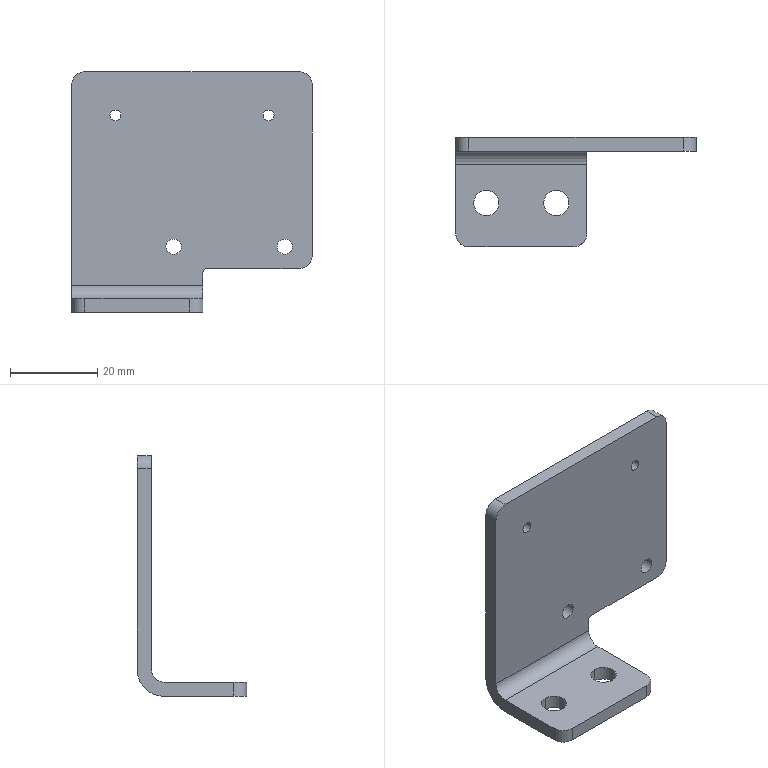Part | STEP file | J014-EBZ05-13-06-Part-1 | 1 solid | 30 faces | box 55 x 25 x 55 mm | volume 10507 mm3 | cylinder 20 | plane 10 | commonest cylinder face diameters 6 x6 2.5 x4 3.5 x4 5.8 x4 2 x1 12 x1
STEP:
#1=CARTESIAN_POINT('',(43.75,0.,45.));
#2=VERTEX_POINT('',#1);
#3=CARTESIAN_POINT('',(46.25,0.,45.));
#4=VERTEX_POINT('',#3);
#5=CARTESIAN_POINT('',(45.,0.,45.));
#6=DIRECTION('',(0.,-1.,0.));
#7=DIRECTION('',(1.,0.,0.));
#8=AXIS2_PLACEMENT_3D('',#5,#6,#7);
#9=CIRCLE('',#8,1.25);
#10=EDGE_CURVE('',#2,#4,#9,.T.);
#11=ORIENTED_EDGE('',*,*,#10,.F.);
#12=CARTESIAN_POINT('',(43.75,-3.2,45.));
#13=VERTEX_POINT('',#12);
#14=CARTESIAN_POINT('',(43.75,0.,45.));
#15=DIRECTION('',(0.,-1.,0.));
#16=VECTOR('',#15,1000.);
#17=LINE('',#14,#16);
#18=EDGE_CURVE('',#2,#13,#17,.T.);
#19=ORIENTED_EDGE('',*,*,#18,.T.);
#20=CARTESIAN_POINT('',(46.25,-3.2,45.));
#21=VERTEX_POINT('',#20);
#22=CARTESIAN_POINT('',(45.,-3.2,45.));
#23=DIRECTION('',(0.,1.,0.));
#24=DIRECTION('',(-1.,0.,0.));
#25=AXIS2_PLACEMENT_3D('',#22,#23,#24);
#26=CIRCLE('',#25,1.25);
#27=EDGE_CURVE('',#21,#13,#26,.T.);
#28=ORIENTED_EDGE('',*,*,#27,.F.);
#29=CARTESIAN_POINT('',(46.25,0.,45.));
#30=DIRECTION('',(0.,-1.,0.));
#31=VECTOR('',#30,1000.);
#32=LINE('',#29,#31);
#33=EDGE_CURVE('',#4,#21,#32,.T.);
#34=ORIENTED_EDGE('',*,*,#33,.F.);
#35=EDGE_LOOP('',(#11,#19,#28,#34));
#36=FACE_OUTER_BOUND('',#35,.T.);
#37=CARTESIAN_POINT('',(45.,0.,45.));
#38=DIRECTION('',(0.,-1.,0.));
#39=DIRECTION('',(1.,0.,0.));
#40=AXIS2_PLACEMENT_3D('',#37,#38,#39);
#41=CYLINDRICAL_SURFACE('',#40,1.25);
#42=ADVANCED_FACE('',(#36),#41,.F.);
#43=CARTESIAN_POINT('',(8.75,0.,45.));
#44=VERTEX_POINT('',#43);
#45=CARTESIAN_POINT('',(11.25,0.,45.));
#46=VERTEX_POINT('',#45);
#47=CARTESIAN_POINT('',(10.,0.,45.));
#48=DIRECTION('',(0.,-1.,0.));
#49=DIRECTION('',(1.,0.,0.));
#50=AXIS2_PLACEMENT_3D('',#47,#48,#49);
#51=CIRCLE('',#50,1.25);
#52=EDGE_CURVE('',#44,#46,#51,.T.);
#53=ORIENTED_EDGE('',*,*,#52,.F.);
#54=CARTESIAN_POINT('',(8.75,-3.2,45.));
#55=VERTEX_POINT('',#54);
#56=CARTESIAN_POINT('',(8.75,0.,45.));
#57=DIRECTION('',(0.,-1.,0.));
#58=VECTOR('',#57,1000.);
#59=LINE('',#56,#58);
#60=EDGE_CURVE('',#44,#55,#59,.T.);
#61=ORIENTED_EDGE('',*,*,#60,.T.);
#62=CARTESIAN_POINT('',(11.25,-3.2,45.));
#63=VERTEX_POINT('',#62);
#64=CARTESIAN_POINT('',(10.,-3.2,45.));
#65=DIRECTION('',(0.,1.,0.));
#66=DIRECTION('',(-1.,0.,0.));
#67=AXIS2_PLACEMENT_3D('',#64,#65,#66);
#68=CIRCLE('',#67,1.25);
#69=EDGE_CURVE('',#63,#55,#68,.T.);
#70=ORIENTED_EDGE('',*,*,#69,.F.);
#71=CARTESIAN_POINT('',(11.25,0.,45.));
#72=DIRECTION('',(0.,-1.,0.));
#73=VECTOR('',#72,1000.);
#74=LINE('',#71,#73);
#75=EDGE_CURVE('',#46,#63,#74,.T.);
#76=ORIENTED_EDGE('',*,*,#75,.F.);
#77=EDGE_LOOP('',(#53,#61,#70,#76));
#78=FACE_OUTER_BOUND('',#77,.T.);
#79=CARTESIAN_POINT('',(10.,0.,45.));
#80=DIRECTION('',(0.,-1.,0.));
#81=DIRECTION('',(1.,0.,0.));
#82=AXIS2_PLACEMENT_3D('',#79,#80,#81);
#83=CYLINDRICAL_SURFACE('',#82,1.25);
#84=ADVANCED_FACE('',(#78),#83,.F.);
#85=CARTESIAN_POINT('',(21.55,0.,15.));
#86=VERTEX_POINT('',#85);
#87=CARTESIAN_POINT('',(25.05,0.,15.));
#88=VERTEX_POINT('',#87);
#89=CARTESIAN_POINT('',(23.3,0.,15.));
#90=DIRECTION('',(0.,-1.,0.));
#91=DIRECTION('',(1.,0.,0.));
#92=AXIS2_PLACEMENT_3D('',#89,#90,#91);
#93=CIRCLE('',#92,1.75);
#94=EDGE_CURVE('',#86,#88,#93,.T.);
#95=ORIENTED_EDGE('',*,*,#94,.F.);
#96=CARTESIAN_POINT('',(21.55,-3.2,15.));
#97=VERTEX_POINT('',#96);
#98=CARTESIAN_POINT('',(21.55,0.,15.));
#99=DIRECTION('',(0.,-1.,0.));
#100=VECTOR('',#99,1000.);
#101=LINE('',#98,#100);
#102=EDGE_CURVE('',#86,#97,#101,.T.);
#103=ORIENTED_EDGE('',*,*,#102,.T.);
#104=CARTESIAN_POINT('',(25.05,-3.2,15.));
#105=VERTEX_POINT('',#104);
#106=CARTESIAN_POINT('',(23.3,-3.2,15.));
#107=DIRECTION('',(0.,1.,0.));
#108=DIRECTION('',(-1.,0.,0.));
#109=AXIS2_PLACEMENT_3D('',#106,#107,#108);
#110=CIRCLE('',#109,1.75);
#111=EDGE_CURVE('',#105,#97,#110,.T.);
#112=ORIENTED_EDGE('',*,*,#111,.F.);
#113=CARTESIAN_POINT('',(25.05,0.,15.));
#114=DIRECTION('',(0.,-1.,0.));
#115=VECTOR('',#114,1000.);
#116=LINE('',#113,#115);
#117=EDGE_CURVE('',#88,#105,#116,.T.);
#118=ORIENTED_EDGE('',*,*,#117,.F.);
#119=EDGE_LOOP('',(#95,#103,#112,#118));
#120=FACE_OUTER_BOUND('',#119,.T.);
#121=CARTESIAN_POINT('',(23.3,0.,15.));
#122=DIRECTION('',(0.,-1.,0.));
#123=DIRECTION('',(1.,0.,0.));
#124=AXIS2_PLACEMENT_3D('',#121,#122,#123);
#125=CYLINDRICAL_SURFACE('',#124,1.75);
#126=ADVANCED_FACE('',(#120),#125,.F.);
#127=CARTESIAN_POINT('',(46.95,0.,15.));
#128=VERTEX_POINT('',#127);
#129=CARTESIAN_POINT('',(50.45,0.,15.));
#130=VERTEX_POINT('',#129);
#131=CARTESIAN_POINT('',(48.7,0.,15.));
#132=DIRECTION('',(0.,-1.,0.));
#133=DIRECTION('',(1.,0.,0.));
#134=AXIS2_PLACEMENT_3D('',#131,#132,#133);
#135=CIRCLE('',#134,1.75);
#136=EDGE_CURVE('',#128,#130,#135,.T.);
#137=ORIENTED_EDGE('',*,*,#136,.F.);
#138=CARTESIAN_POINT('',(46.95,-3.2,15.));
#139=VERTEX_POINT('',#138);
#140=CARTESIAN_POINT('',(46.95,0.,15.));
#141=DIRECTION('',(0.,-1.,0.));
#142=VECTOR('',#141,1000.);
#143=LINE('',#140,#142);
#144=EDGE_CURVE('',#128,#139,#143,.T.);
#145=ORIENTED_EDGE('',*,*,#144,.T.);
#146=CARTESIAN_POINT('',(50.45,-3.2,15.));
#147=VERTEX_POINT('',#146);
#148=CARTESIAN_POINT('',(48.7,-3.2,15.));
#149=DIRECTION('',(0.,1.,0.));
#150=DIRECTION('',(-1.,0.,0.));
#151=AXIS2_PLACEMENT_3D('',#148,#149,#150);
#152=CIRCLE('',#151,1.75);
#153=EDGE_CURVE('',#147,#139,#152,.T.);
#154=ORIENTED_EDGE('',*,*,#153,.F.);
#155=CARTESIAN_POINT('',(50.45,0.,15.));
#156=DIRECTION('',(0.,-1.,0.));
#157=VECTOR('',#156,1000.);
#158=LINE('',#155,#157);
#159=EDGE_CURVE('',#130,#147,#158,.T.);
#160=ORIENTED_EDGE('',*,*,#159,.F.);
#161=EDGE_LOOP('',(#137,#145,#154,#160));
#162=FACE_OUTER_BOUND('',#161,.T.);
#163=CARTESIAN_POINT('',(48.7,0.,15.));
#164=DIRECTION('',(0.,-1.,0.));
#165=DIRECTION('',(1.,0.,0.));
#166=AXIS2_PLACEMENT_3D('',#163,#164,#165);
#167=CYLINDRICAL_SURFACE('',#166,1.75);
#168=ADVANCED_FACE('',(#162),#167,.F.);
#169=CARTESIAN_POINT('',(7.,-17.9,3.2));
#170=VERTEX_POINT('',#169);
#171=CARTESIAN_POINT('',(7.,-12.1,3.2));
#172=VERTEX_POINT('',#171);
#173=CARTESIAN_POINT('',(7.,-15.,3.2));
#174=DIRECTION('',(0.,0.,-1.));
#175=DIRECTION('',(0.,1.,0.));
#176=AXIS2_PLACEMENT_3D('',#173,#174,#175);
#177=CIRCLE('',#176,2.9);
#178=EDGE_CURVE('',#170,#172,#177,.T.);
#179=ORIENTED_EDGE('',*,*,#178,.F.);
#180=CARTESIAN_POINT('',(7.,-17.9,0.));
#181=VERTEX_POINT('',#180);
#182=CARTESIAN_POINT('',(7.,-17.9,3.2));
#183=DIRECTION('',(0.,0.,-1.));
#184=VECTOR('',#183,1000.);
#185=LINE('',#182,#184);
#186=EDGE_CURVE('',#170,#181,#185,.T.);
#187=ORIENTED_EDGE('',*,*,#186,.T.);
#188=CARTESIAN_POINT('',(7.,-12.1,0.));
#189=VERTEX_POINT('',#188);
#190=CARTESIAN_POINT('',(7.,-15.,0.));
#191=DIRECTION('',(0.,0.,-1.));
#192=DIRECTION('',(0.,1.,0.));
#193=AXIS2_PLACEMENT_3D('',#190,#191,#192);
#194=CIRCLE('',#193,2.9);
#195=EDGE_CURVE('',#181,#189,#194,.T.);
#196=ORIENTED_EDGE('',*,*,#195,.T.);
#197=CARTESIAN_POINT('',(7.,-12.1,3.2));
#198=DIRECTION('',(0.,0.,-1.));
#199=VECTOR('',#198,1000.);
#200=LINE('',#197,#199);
#201=EDGE_CURVE('',#172,#189,#200,.T.);
#202=ORIENTED_EDGE('',*,*,#201,.F.);
#203=EDGE_LOOP('',(#179,#187,#196,#202));
#204=FACE_OUTER_BOUND('',#203,.T.);
#205=CARTESIAN_POINT('',(7.,-15.,3.2));
#206=DIRECTION('',(0.,0.,-1.));
#207=DIRECTION('',(0.,1.,0.));
#208=AXIS2_PLACEMENT_3D('',#205,#206,#207);
#209=CYLINDRICAL_SURFACE('',#208,2.9);
#210=ADVANCED_FACE('',(#204),#209,.F.);
#211=CARTESIAN_POINT('',(23.,-17.9,3.2));
#212=VERTEX_POINT('',#211);
#213=CARTESIAN_POINT('',(23.,-12.1,3.2));
#214=VERTEX_POINT('',#213);
#215=CARTESIAN_POINT('',(23.,-15.,3.2));
#216=DIRECTION('',(0.,0.,-1.));
#217=DIRECTION('',(0.,1.,0.));
#218=AXIS2_PLACEMENT_3D('',#215,#216,#217);
#219=CIRCLE('',#218,2.9);
#220=EDGE_CURVE('',#212,#214,#219,.T.);
#221=ORIENTED_EDGE('',*,*,#220,.F.);
#222=CARTESIAN_POINT('',(23.,-17.9,0.));
#223=VERTEX_POINT('',#222);
#224=CARTESIAN_POINT('',(23.,-17.9,3.2));
#225=DIRECTION('',(0.,0.,-1.));
#226=VECTOR('',#225,1000.);
#227=LINE('',#224,#226);
#228=EDGE_CURVE('',#212,#223,#227,.T.);
#229=ORIENTED_EDGE('',*,*,#228,.T.);
#230=CARTESIAN_POINT('',(23.,-12.1,0.));
#231=VERTEX_POINT('',#230);
#232=CARTESIAN_POINT('',(23.,-15.,0.));
#233=DIRECTION('',(0.,0.,-1.));
#234=DIRECTION('',(0.,1.,0.));
#235=AXIS2_PLACEMENT_3D('',#232,#233,#234);
#236=CIRCLE('',#235,2.9);
#237=EDGE_CURVE('',#223,#231,#236,.T.);
#238=ORIENTED_EDGE('',*,*,#237,.T.);
#239=CARTESIAN_POINT('',(23.,-12.1,3.2));
#240=DIRECTION('',(0.,0.,-1.));
#241=VECTOR('',#240,1000.);
#242=LINE('',#239,#241);
#243=EDGE_CURVE('',#214,#231,#242,.T.);
#244=ORIENTED_EDGE('',*,*,#243,.F.);
#245=EDGE_LOOP('',(#221,#229,#238,#244));
#246=FACE_OUTER_BOUND('',#245,.T.);
#247=CARTESIAN_POINT('',(23.,-15.,3.2));
#248=DIRECTION('',(0.,0.,-1.));
#249=DIRECTION('',(0.,1.,0.));
#250=AXIS2_PLACEMENT_3D('',#247,#248,#249);
#251=CYLINDRICAL_SURFACE('',#250,2.9);
#252=ADVANCED_FACE('',(#246),#251,.F.);
#253=CARTESIAN_POINT('',(7.,-15.,3.2));
#254=DIRECTION('',(0.,0.,-1.));
#255=DIRECTION('',(0.,1.,0.));
#256=AXIS2_PLACEMENT_3D('',#253,#254,#255);
#257=CIRCLE('',#256,2.9);
#258=EDGE_CURVE('',#172,#170,#257,.T.);
#259=ORIENTED_EDGE('',*,*,#258,.T.);
#260=ORIENTED_EDGE('',*,*,#178,.T.);
#261=EDGE_LOOP('',(#259,#260));
#262=FACE_BOUND('',#261,.T.);
#263=CARTESIAN_POINT('',(23.,-15.,3.2));
#264=DIRECTION('',(0.,0.,-1.));
#265=DIRECTION('',(0.,1.,0.));
#266=AXIS2_PLACEMENT_3D('',#263,#264,#265);
#267=CIRCLE('',#266,2.9);
#268=EDGE_CURVE('',#214,#212,#267,.T.);
#269=ORIENTED_EDGE('',*,*,#268,.T.);
#270=ORIENTED_EDGE('',*,*,#220,.T.);
#271=EDGE_LOOP('',(#269,#270));
#272=FACE_BOUND('',#271,.T.);
#273=CARTESIAN_POINT('',(27.,-25.,3.2));
#274=VERTEX_POINT('',#273);
#275=CARTESIAN_POINT('',(3.,-25.,3.2));
#276=VERTEX_POINT('',#275);
#277=CARTESIAN_POINT('',(15.,-25.,3.2));
#278=DIRECTION('',(-1.,0.,0.));
#279=VECTOR('',#278,1000.);
#280=LINE('',#277,#279);
#281=EDGE_CURVE('',#274,#276,#280,.T.);
#282=ORIENTED_EDGE('',*,*,#281,.F.);
#283=CARTESIAN_POINT('',(30.,-22.,3.2));
#284=VERTEX_POINT('',#283);
#285=CARTESIAN_POINT('',(27.,-22.,3.2));
#286=DIRECTION('',(0.,0.,1.));
#287=DIRECTION('',(0.,-1.,0.));
#288=AXIS2_PLACEMENT_3D('',#285,#286,#287);
#289=CIRCLE('',#288,3.);
#290=EDGE_CURVE('',#274,#284,#289,.T.);
#291=ORIENTED_EDGE('',*,*,#290,.T.);
#292=CARTESIAN_POINT('',(30.,-6.2,3.2));
#293=VERTEX_POINT('',#292);
#294=CARTESIAN_POINT('',(30.,-12.5,3.2));
#295=DIRECTION('',(0.,-1.,0.));
#296=VECTOR('',#295,1000.);
#297=LINE('',#294,#296);
#298=EDGE_CURVE('',#293,#284,#297,.T.);
#299=ORIENTED_EDGE('',*,*,#298,.F.);
#300=CARTESIAN_POINT('',(0.,-6.2,3.2));
#301=VERTEX_POINT('',#300);
#302=CARTESIAN_POINT('',(0.,-6.2,3.2));
#303=DIRECTION('',(-1.,0.,0.));
#304=VECTOR('',#303,1000.);
#305=LINE('',#302,#304);
#306=EDGE_CURVE('',#293,#301,#305,.T.);
#307=ORIENTED_EDGE('',*,*,#306,.T.);
#308=CARTESIAN_POINT('',(0.,-22.,3.2));
#309=VERTEX_POINT('',#308);
#310=CARTESIAN_POINT('',(0.,-12.5,3.2));
#311=DIRECTION('',(0.,1.,0.));
#312=VECTOR('',#311,1000.);
#313=LINE('',#310,#312);
#314=EDGE_CURVE('',#309,#301,#313,.T.);
#315=ORIENTED_EDGE('',*,*,#314,.F.);
#316=CARTESIAN_POINT('',(3.,-22.,3.2));
#317=DIRECTION('',(0.,0.,1.));
#318=DIRECTION('',(0.,-1.,0.));
#319=AXIS2_PLACEMENT_3D('',#316,#317,#318);
#320=CIRCLE('',#319,3.);
#321=EDGE_CURVE('',#309,#276,#320,.T.);
#322=ORIENTED_EDGE('',*,*,#321,.T.);
#323=EDGE_LOOP('',(#282,#291,#299,#307,#315,#322));
#324=FACE_OUTER_BOUND('',#323,.T.);
#325=CARTESIAN_POINT('',(15.,-12.5,3.2));
#326=DIRECTION('',(0.,0.,1.));
#327=DIRECTION('',(0.,-1.,0.));
#328=AXIS2_PLACEMENT_3D('',#325,#326,#327);
#329=PLANE('',#328);
#330=ADVANCED_FACE('',(#262,#272,#324),#329,.T.);
#331=CARTESIAN_POINT('',(0.,-3.2,6.2));
#332=VERTEX_POINT('',#331);
#333=CARTESIAN_POINT('',(0.,-3.2,52.));
#334=VERTEX_POINT('',#333);
#335=CARTESIAN_POINT('',(0.,-3.2,3.2));
#336=DIRECTION('',(0.,0.,1.));
#337=VECTOR('',#336,1000.);
#338=LINE('',#335,#337);
#339=EDGE_CURVE('',#332,#334,#338,.T.);
#340=ORIENTED_EDGE('',*,*,#339,.T.);
#341=CARTESIAN_POINT('',(0.,0.,52.));
#342=VERTEX_POINT('',#341);
#343=CARTESIAN_POINT('',(0.,-12.5,52.));
#344=DIRECTION('',(0.,1.,0.));
#345=VECTOR('',#344,1000.);
#346=LINE('',#343,#345);
#347=EDGE_CURVE('',#334,#342,#346,.T.);
#348=ORIENTED_EDGE('',*,*,#347,.T.);
#349=CARTESIAN_POINT('',(0.,0.,6.));
#350=VERTEX_POINT('',#349);
#351=CARTESIAN_POINT('',(0.,0.,0.));
#352=DIRECTION('',(0.,0.,1.));
#353=VECTOR('',#352,1000.);
#354=LINE('',#351,#353);
#355=EDGE_CURVE('',#350,#342,#354,.T.);
#356=ORIENTED_EDGE('',*,*,#355,.F.);
#357=CARTESIAN_POINT('',(0.,-6.,0.));
#358=VERTEX_POINT('',#357);
#359=CARTESIAN_POINT('',(0.,-6.,6.));
#360=DIRECTION('',(-1.,0.,0.));
#361=DIRECTION('',(0.,0.,-1.));
#362=AXIS2_PLACEMENT_3D('',#359,#360,#361);
#363=CIRCLE('',#362,6.);
#364=EDGE_CURVE('',#350,#358,#363,.T.);
#365=ORIENTED_EDGE('',*,*,#364,.T.);
#366=CARTESIAN_POINT('',(0.,-22.,0.));
#367=VERTEX_POINT('',#366);
#368=CARTESIAN_POINT('',(0.,-12.5,0.));
#369=DIRECTION('',(0.,-1.,0.));
#370=VECTOR('',#369,1000.);
#371=LINE('',#368,#370);
#372=EDGE_CURVE('',#358,#367,#371,.T.);
#373=ORIENTED_EDGE('',*,*,#372,.T.);
#374=CARTESIAN_POINT('',(0.,-22.,0.));
#375=DIRECTION('',(0.,0.,1.));
#376=VECTOR('',#375,1000.);
#377=LINE('',#374,#376);
#378=EDGE_CURVE('',#367,#309,#377,.T.);
#379=ORIENTED_EDGE('',*,*,#378,.T.);
#380=ORIENTED_EDGE('',*,*,#314,.T.);
#381=CARTESIAN_POINT('',(0.,-6.2,6.2));
#382=DIRECTION('',(1.,0.,0.));
#383=DIRECTION('',(0.,0.,-1.));
#384=AXIS2_PLACEMENT_3D('',#381,#382,#383);
#385=CIRCLE('',#384,3.);
#386=EDGE_CURVE('',#301,#332,#385,.T.);
#387=ORIENTED_EDGE('',*,*,#386,.T.);
#388=EDGE_LOOP('',(#340,#348,#356,#365,#373,#379,#380,#387));
#389=FACE_OUTER_BOUND('',#388,.T.);
#390=CARTESIAN_POINT('',(0.,-12.5,0.));
#391=DIRECTION('',(-1.,0.,0.));
#392=DIRECTION('',(0.,0.,-1.));
#393=AXIS2_PLACEMENT_3D('',#390,#391,#392);
#394=PLANE('',#393);
#395=ADVANCED_FACE('',(#389),#394,.T.);
#396=CARTESIAN_POINT('',(45.,0.,45.));
#397=DIRECTION('',(0.,-1.,0.));
#398=DIRECTION('',(1.,0.,0.));
#399=AXIS2_PLACEMENT_3D('',#396,#397,#398);
#400=CIRCLE('',#399,1.25);
#401=EDGE_CURVE('',#4,#2,#400,.T.);
#402=ORIENTED_EDGE('',*,*,#401,.T.);
#403=ORIENTED_EDGE('',*,*,#10,.T.);
#404=EDGE_LOOP('',(#402,#403));
#405=FACE_BOUND('',#404,.T.);
#406=CARTESIAN_POINT('',(10.,0.,45.));
#407=DIRECTION('',(0.,-1.,0.));
#408=DIRECTION('',(1.,0.,0.));
#409=AXIS2_PLACEMENT_3D('',#406,#407,#408);
#410=CIRCLE('',#409,1.25);
#411=EDGE_CURVE('',#46,#44,#410,.T.);
#412=ORIENTED_EDGE('',*,*,#411,.T.);
#413=ORIENTED_EDGE('',*,*,#52,.T.);
#414=EDGE_LOOP('',(#412,#413));
#415=FACE_BOUND('',#414,.T.);
#416=CARTESIAN_POINT('',(23.3,0.,15.));
#417=DIRECTION('',(0.,-1.,0.));
#418=DIRECTION('',(1.,0.,0.));
#419=AXIS2_PLACEMENT_3D('',#416,#417,#418);
#420=CIRCLE('',#419,1.75);
#421=EDGE_CURVE('',#88,#86,#420,.T.);
#422=ORIENTED_EDGE('',*,*,#421,.T.);
#423=ORIENTED_EDGE('',*,*,#94,.T.);
#424=EDGE_LOOP('',(#422,#423));
#425=FACE_BOUND('',#424,.T.);
#426=CARTESIAN_POINT('',(48.7,0.,15.));
#427=DIRECTION('',(0.,-1.,0.));
#428=DIRECTION('',(1.,0.,0.));
#429=AXIS2_PLACEMENT_3D('',#426,#427,#428);
#430=CIRCLE('',#429,1.75);
#431=EDGE_CURVE('',#130,#128,#430,.T.);
#432=ORIENTED_EDGE('',*,*,#431,.T.);
#433=ORIENTED_EDGE('',*,*,#136,.T.);
#434=EDGE_LOOP('',(#432,#433));
#435=FACE_BOUND('',#434,.T.);
#436=CARTESIAN_POINT('',(55.,0.,13.));
#437=VERTEX_POINT('',#436);
#438=CARTESIAN_POINT('',(55.,0.,52.));
#439=VERTEX_POINT('',#438);
#440=CARTESIAN_POINT('',(55.,0.,32.5));
#441=DIRECTION('',(0.,0.,1.));
#442=VECTOR('',#441,1000.);
#443=LINE('',#440,#442);
#444=EDGE_CURVE('',#437,#439,#443,.T.);
#445=ORIENTED_EDGE('',*,*,#444,.F.);
#446=CARTESIAN_POINT('',(52.,0.,10.));
#447=VERTEX_POINT('',#446);
#448=CARTESIAN_POINT('',(52.,0.,13.));
#449=DIRECTION('',(0.,1.,0.));
#450=DIRECTION('',(0.,0.,1.));
#451=AXIS2_PLACEMENT_3D('',#448,#449,#450);
#452=CIRCLE('',#451,3.);
#453=EDGE_CURVE('',#437,#447,#452,.T.);
#454=ORIENTED_EDGE('',*,*,#453,.T.);
#455=CARTESIAN_POINT('',(31.,0.,10.));
#456=VERTEX_POINT('',#455);
#457=CARTESIAN_POINT('',(42.5,0.,10.));
#458=DIRECTION('',(1.,0.,0.));
#459=VECTOR('',#458,1000.);
#460=LINE('',#457,#459);
#461=EDGE_CURVE('',#456,#447,#460,.T.);
#462=ORIENTED_EDGE('',*,*,#461,.F.);
#463=CARTESIAN_POINT('',(30.,0.,9.));
#464=VERTEX_POINT('',#463);
#465=CARTESIAN_POINT('',(31.,0.,9.));
#466=DIRECTION('',(0.,-1.,0.));
#467=DIRECTION('',(0.,0.,1.));
#468=AXIS2_PLACEMENT_3D('',#465,#466,#467);
#469=CIRCLE('',#468,1.);
#470=EDGE_CURVE('',#456,#464,#469,.T.);
#471=ORIENTED_EDGE('',*,*,#470,.T.);
#472=CARTESIAN_POINT('',(30.,0.,6.));
#473=VERTEX_POINT('',#472);
#474=CARTESIAN_POINT('',(30.,0.,0.));
#475=DIRECTION('',(0.,0.,1.));
#476=VECTOR('',#475,1000.);
#477=LINE('',#474,#476);
#478=EDGE_CURVE('',#473,#464,#477,.T.);
#479=ORIENTED_EDGE('',*,*,#478,.F.);
#480=CARTESIAN_POINT('',(15.,0.,6.));
#481=DIRECTION('',(-1.,0.,0.));
#482=VECTOR('',#481,1000.);
#483=LINE('',#480,#482);
#484=EDGE_CURVE('',#473,#350,#483,.T.);
#485=ORIENTED_EDGE('',*,*,#484,.T.);
#486=ORIENTED_EDGE('',*,*,#355,.T.);
#487=CARTESIAN_POINT('',(3.,0.,55.));
#488=VERTEX_POINT('',#487);
#489=CARTESIAN_POINT('',(3.,0.,52.));
#490=DIRECTION('',(0.,1.,0.));
#491=DIRECTION('',(0.,0.,1.));
#492=AXIS2_PLACEMENT_3D('',#489,#490,#491);
#493=CIRCLE('',#492,3.);
#494=EDGE_CURVE('',#342,#488,#493,.T.);
#495=ORIENTED_EDGE('',*,*,#494,.T.);
#496=CARTESIAN_POINT('',(52.,0.,55.));
#497=VERTEX_POINT('',#496);
#498=CARTESIAN_POINT('',(15.,0.,55.));
#499=DIRECTION('',(1.,0.,0.));
#500=VECTOR('',#499,1000.);
#501=LINE('',#498,#500);
#502=EDGE_CURVE('',#488,#497,#501,.T.);
#503=ORIENTED_EDGE('',*,*,#502,.T.);
#504=CARTESIAN_POINT('',(52.,0.,52.));
#505=DIRECTION('',(0.,1.,0.));
#506=DIRECTION('',(0.,0.,1.));
#507=AXIS2_PLACEMENT_3D('',#504,#505,#506);
#508=CIRCLE('',#507,3.);
#509=EDGE_CURVE('',#497,#439,#508,.T.);
#510=ORIENTED_EDGE('',*,*,#509,.T.);
#511=EDGE_LOOP('',(#445,#454,#462,#471,#479,#485,#486,#495,#503,#510));
#512=FACE_OUTER_BOUND('',#511,.T.);
#513=CARTESIAN_POINT('',(15.,0.,0.));
#514=DIRECTION('',(0.,1.,0.));
#515=DIRECTION('',(0.,0.,1.));
#516=AXIS2_PLACEMENT_3D('',#513,#514,#515);
#517=PLANE('',#516);
#518=ADVANCED_FACE('',(#405,#415,#425,#435,#512),#517,.T.);
#519=ORIENTED_EDGE('',*,*,#478,.T.);
#520=CARTESIAN_POINT('',(30.,-3.2,9.));
#521=VERTEX_POINT('',#520);
#522=CARTESIAN_POINT('',(30.,-3.2,9.));
#523=DIRECTION('',(0.,-1.,0.));
#524=VECTOR('',#523,1000.);
#525=LINE('',#522,#524);
#526=EDGE_CURVE('',#464,#521,#525,.T.);
#527=ORIENTED_EDGE('',*,*,#526,.T.);
#528=CARTESIAN_POINT('',(30.,-3.2,6.2));
#529=VERTEX_POINT('',#528);
#530=CARTESIAN_POINT('',(30.,-3.2,3.2));
#531=DIRECTION('',(0.,0.,1.));
#532=VECTOR('',#531,1000.);
#533=LINE('',#530,#532);
#534=EDGE_CURVE('',#529,#521,#533,.T.);
#535=ORIENTED_EDGE('',*,*,#534,.F.);
#536=CARTESIAN_POINT('',(30.,-6.2,6.2));
#537=DIRECTION('',(-1.,0.,0.));
#538=DIRECTION('',(0.,0.,1.));
#539=AXIS2_PLACEMENT_3D('',#536,#537,#538);
#540=CIRCLE('',#539,3.);
#541=EDGE_CURVE('',#529,#293,#540,.T.);
#542=ORIENTED_EDGE('',*,*,#541,.T.);
#543=ORIENTED_EDGE('',*,*,#298,.T.);
#544=CARTESIAN_POINT('',(30.,-22.,0.));
#545=VERTEX_POINT('',#544);
#546=CARTESIAN_POINT('',(30.,-22.,0.));
#547=DIRECTION('',(0.,0.,-1.));
#548=VECTOR('',#547,1000.);
#549=LINE('',#546,#548);
#550=EDGE_CURVE('',#284,#545,#549,.T.);
#551=ORIENTED_EDGE('',*,*,#550,.T.);
#552=CARTESIAN_POINT('',(30.,-6.,0.));
#553=VERTEX_POINT('',#552);
#554=CARTESIAN_POINT('',(30.,-12.5,0.));
#555=DIRECTION('',(0.,1.,0.));
#556=VECTOR('',#555,1000.);
#557=LINE('',#554,#556);
#558=EDGE_CURVE('',#545,#553,#557,.T.);
#559=ORIENTED_EDGE('',*,*,#558,.T.);
#560=CARTESIAN_POINT('',(30.,-6.,6.));
#561=DIRECTION('',(1.,0.,0.));
#562=DIRECTION('',(0.,0.,1.));
#563=AXIS2_PLACEMENT_3D('',#560,#561,#562);
#564=CIRCLE('',#563,6.);
#565=EDGE_CURVE('',#553,#473,#564,.T.);
#566=ORIENTED_EDGE('',*,*,#565,.T.);
#567=EDGE_LOOP('',(#519,#527,#535,#542,#543,#551,#559,#566));
#568=FACE_OUTER_BOUND('',#567,.T.);
#569=CARTESIAN_POINT('',(30.,-12.5,0.));
#570=DIRECTION('',(1.,0.,0.));
#571=DIRECTION('',(0.,0.,1.));
#572=AXIS2_PLACEMENT_3D('',#569,#570,#571);
#573=PLANE('',#572);
#574=ADVANCED_FACE('',(#568),#573,.T.);
#575=CARTESIAN_POINT('',(7.,-15.,0.));
#576=DIRECTION('',(0.,0.,-1.));
#577=DIRECTION('',(0.,1.,0.));
#578=AXIS2_PLACEMENT_3D('',#575,#576,#577);
#579=CIRCLE('',#578,2.9);
#580=EDGE_CURVE('',#189,#181,#579,.T.);
#581=ORIENTED_EDGE('',*,*,#580,.F.);
#582=ORIENTED_EDGE('',*,*,#195,.F.);
#583=EDGE_LOOP('',(#581,#582));
#584=FACE_BOUND('',#583,.T.);
#585=CARTESIAN_POINT('',(23.,-15.,0.));
#586=DIRECTION('',(0.,0.,-1.));
#587=DIRECTION('',(0.,1.,0.));
#588=AXIS2_PLACEMENT_3D('',#585,#586,#587);
#589=CIRCLE('',#588,2.9);
#590=EDGE_CURVE('',#231,#223,#589,.T.);
#591=ORIENTED_EDGE('',*,*,#590,.F.);
#592=ORIENTED_EDGE('',*,*,#237,.F.);
#593=EDGE_LOOP('',(#591,#592));
#594=FACE_BOUND('',#593,.T.);
#595=ORIENTED_EDGE('',*,*,#558,.F.);
#596=CARTESIAN_POINT('',(27.,-25.,0.));
#597=VERTEX_POINT('',#596);
#598=CARTESIAN_POINT('',(27.,-22.,0.));
#599=DIRECTION('',(0.,0.,-1.));
#600=DIRECTION('',(0.,1.,0.));
#601=AXIS2_PLACEMENT_3D('',#598,#599,#600);
#602=CIRCLE('',#601,3.);
#603=EDGE_CURVE('',#545,#597,#602,.T.);
#604=ORIENTED_EDGE('',*,*,#603,.T.);
#605=CARTESIAN_POINT('',(3.,-25.,0.));
#606=VERTEX_POINT('',#605);
#607=CARTESIAN_POINT('',(15.,-25.,0.));
#608=DIRECTION('',(1.,0.,0.));
#609=VECTOR('',#608,1000.);
#610=LINE('',#607,#609);
#611=EDGE_CURVE('',#606,#597,#610,.T.);
#612=ORIENTED_EDGE('',*,*,#611,.F.);
#613=CARTESIAN_POINT('',(3.,-22.,0.));
#614=DIRECTION('',(0.,0.,-1.));
#615=DIRECTION('',(0.,1.,0.));
#616=AXIS2_PLACEMENT_3D('',#613,#614,#615);
#617=CIRCLE('',#616,3.);
#618=EDGE_CURVE('',#606,#367,#617,.T.);
#619=ORIENTED_EDGE('',*,*,#618,.T.);
#620=ORIENTED_EDGE('',*,*,#372,.F.);
#621=CARTESIAN_POINT('',(15.,-6.,0.));
#622=DIRECTION('',(1.,0.,0.));
#623=VECTOR('',#622,1000.);
#624=LINE('',#621,#623);
#625=EDGE_CURVE('',#358,#553,#624,.T.);
#626=ORIENTED_EDGE('',*,*,#625,.T.);
#627=EDGE_LOOP('',(#595,#604,#612,#619,#620,#626));
#628=FACE_OUTER_BOUND('',#627,.T.);
#629=CARTESIAN_POINT('',(15.,-12.5,0.));
#630=DIRECTION('',(0.,0.,-1.));
#631=DIRECTION('',(0.,1.,0.));
#632=AXIS2_PLACEMENT_3D('',#629,#630,#631);
#633=PLANE('',#632);
#634=ADVANCED_FACE('',(#584,#594,#628),#633,.T.);
#635=ORIENTED_EDGE('',*,*,#611,.T.);
#636=CARTESIAN_POINT('',(27.,-25.,0.));
#637=DIRECTION('',(0.,0.,1.));
#638=VECTOR('',#637,1000.);
#639=LINE('',#636,#638);
#640=EDGE_CURVE('',#597,#274,#639,.T.);
#641=ORIENTED_EDGE('',*,*,#640,.T.);
#642=ORIENTED_EDGE('',*,*,#281,.T.);
#643=CARTESIAN_POINT('',(3.,-25.,0.));
#644=DIRECTION('',(0.,0.,-1.));
#645=VECTOR('',#644,1000.);
#646=LINE('',#643,#645);
#647=EDGE_CURVE('',#276,#606,#646,.T.);
#648=ORIENTED_EDGE('',*,*,#647,.T.);
#649=EDGE_LOOP('',(#635,#641,#642,#648));
#650=FACE_OUTER_BOUND('',#649,.T.);
#651=CARTESIAN_POINT('',(15.,-25.,0.));
#652=DIRECTION('',(0.,-1.,0.));
#653=DIRECTION('',(0.,0.,-1.));
#654=AXIS2_PLACEMENT_3D('',#651,#652,#653);
#655=PLANE('',#654);
#656=ADVANCED_FACE('',(#650),#655,.T.);
#657=CARTESIAN_POINT('',(52.,-3.2,55.));
#658=VERTEX_POINT('',#657);
#659=CARTESIAN_POINT('',(3.,-3.2,55.));
#660=VERTEX_POINT('',#659);
#661=CARTESIAN_POINT('',(15.,-3.2,55.));
#662=DIRECTION('',(-1.,0.,0.));
#663=VECTOR('',#662,1000.);
#664=LINE('',#661,#663);
#665=EDGE_CURVE('',#658,#660,#664,.T.);
#666=ORIENTED_EDGE('',*,*,#665,.F.);
#667=CARTESIAN_POINT('',(52.,-1.6,55.));
#668=DIRECTION('',(0.,1.,0.));
#669=VECTOR('',#668,1000.);
#670=LINE('',#667,#669);
#671=EDGE_CURVE('',#658,#497,#670,.T.);
#672=ORIENTED_EDGE('',*,*,#671,.T.);
#673=ORIENTED_EDGE('',*,*,#502,.F.);
#674=CARTESIAN_POINT('',(3.,-1.6,55.));
#675=DIRECTION('',(0.,-1.,0.));
#676=VECTOR('',#675,1000.);
#677=LINE('',#674,#676);
#678=EDGE_CURVE('',#488,#660,#677,.T.);
#679=ORIENTED_EDGE('',*,*,#678,.T.);
#680=EDGE_LOOP('',(#666,#672,#673,#679));
#681=FACE_OUTER_BOUND('',#680,.T.);
#682=CARTESIAN_POINT('',(15.,-1.6,55.));
#683=DIRECTION('',(0.,0.,1.));
#684=DIRECTION('',(0.,1.,0.));
#685=AXIS2_PLACEMENT_3D('',#682,#683,#684);
#686=PLANE('',#685);
#687=ADVANCED_FACE('',(#681),#686,.T.);
#688=ORIENTED_EDGE('',*,*,#27,.T.);
#689=CARTESIAN_POINT('',(45.,-3.2,45.));
#690=DIRECTION('',(0.,1.,0.));
#691=DIRECTION('',(-1.,0.,0.));
#692=AXIS2_PLACEMENT_3D('',#689,#690,#691);
#693=CIRCLE('',#692,1.25);
#694=EDGE_CURVE('',#13,#21,#693,.T.);
#695=ORIENTED_EDGE('',*,*,#694,.T.);
#696=EDGE_LOOP('',(#688,#695));
#697=FACE_BOUND('',#696,.T.);
#698=ORIENTED_EDGE('',*,*,#69,.T.);
#699=CARTESIAN_POINT('',(10.,-3.2,45.));
#700=DIRECTION('',(0.,1.,0.));
#701=DIRECTION('',(-1.,0.,0.));
#702=AXIS2_PLACEMENT_3D('',#699,#700,#701);
#703=CIRCLE('',#702,1.25);
#704=EDGE_CURVE('',#55,#63,#703,.T.);
#705=ORIENTED_EDGE('',*,*,#704,.T.);
#706=EDGE_LOOP('',(#698,#705));
#707=FACE_BOUND('',#706,.T.);
#708=ORIENTED_EDGE('',*,*,#111,.T.);
#709=CARTESIAN_POINT('',(23.3,-3.2,15.));
#710=DIRECTION('',(0.,1.,0.));
#711=DIRECTION('',(-1.,0.,0.));
#712=AXIS2_PLACEMENT_3D('',#709,#710,#711);
#713=CIRCLE('',#712,1.75);
#714=EDGE_CURVE('',#97,#105,#713,.T.);
#715=ORIENTED_EDGE('',*,*,#714,.T.);
#716=EDGE_LOOP('',(#708,#715));
#717=FACE_BOUND('',#716,.T.);
#718=ORIENTED_EDGE('',*,*,#153,.T.);
#719=CARTESIAN_POINT('',(48.7,-3.2,15.));
#720=DIRECTION('',(0.,1.,0.));
#721=DIRECTION('',(-1.,0.,0.));
#722=AXIS2_PLACEMENT_3D('',#719,#720,#721);
#723=CIRCLE('',#722,1.75);
#724=EDGE_CURVE('',#139,#147,#723,.T.);
#725=ORIENTED_EDGE('',*,*,#724,.T.);
#726=EDGE_LOOP('',(#718,#725));
#727=FACE_BOUND('',#726,.T.);
#728=CARTESIAN_POINT('',(52.,-3.2,10.));
#729=VERTEX_POINT('',#728);
#730=CARTESIAN_POINT('',(31.,-3.2,10.));
#731=VERTEX_POINT('',#730);
#732=CARTESIAN_POINT('',(42.5,-3.2,10.));
#733=DIRECTION('',(-1.,0.,0.));
#734=VECTOR('',#733,1000.);
#735=LINE('',#732,#734);
#736=EDGE_CURVE('',#729,#731,#735,.T.);
#737=ORIENTED_EDGE('',*,*,#736,.F.);
#738=CARTESIAN_POINT('',(55.,-3.2,13.));
#739=VERTEX_POINT('',#738);
#740=CARTESIAN_POINT('',(52.,-3.2,13.));
#741=DIRECTION('',(0.,-1.,0.));
#742=DIRECTION('',(0.,0.,-1.));
#743=AXIS2_PLACEMENT_3D('',#740,#741,#742);
#744=CIRCLE('',#743,3.);
#745=EDGE_CURVE('',#729,#739,#744,.T.);
#746=ORIENTED_EDGE('',*,*,#745,.T.);
#747=CARTESIAN_POINT('',(55.,-3.2,52.));
#748=VERTEX_POINT('',#747);
#749=CARTESIAN_POINT('',(55.,-3.2,32.5));
#750=DIRECTION('',(0.,0.,-1.));
#751=VECTOR('',#750,1000.);
#752=LINE('',#749,#751);
#753=EDGE_CURVE('',#748,#739,#752,.T.);
#754=ORIENTED_EDGE('',*,*,#753,.F.);
#755=CARTESIAN_POINT('',(52.,-3.2,52.));
#756=DIRECTION('',(0.,-1.,0.));
#757=DIRECTION('',(0.,0.,-1.));
#758=AXIS2_PLACEMENT_3D('',#755,#756,#757);
#759=CIRCLE('',#758,3.);
#760=EDGE_CURVE('',#748,#658,#759,.T.);
#761=ORIENTED_EDGE('',*,*,#760,.T.);
#762=ORIENTED_EDGE('',*,*,#665,.T.);
#763=CARTESIAN_POINT('',(3.,-3.2,52.));
#764=DIRECTION('',(0.,-1.,0.));
#765=DIRECTION('',(0.,0.,-1.));
#766=AXIS2_PLACEMENT_3D('',#763,#764,#765);
#767=CIRCLE('',#766,3.);
#768=EDGE_CURVE('',#660,#334,#767,.T.);
#769=ORIENTED_EDGE('',*,*,#768,.T.);
#770=ORIENTED_EDGE('',*,*,#339,.F.);
#771=CARTESIAN_POINT('',(30.,-3.2,6.2));
#772=DIRECTION('',(1.,0.,0.));
#773=VECTOR('',#772,1000.);
#774=LINE('',#771,#773);
#775=EDGE_CURVE('',#332,#529,#774,.T.);
#776=ORIENTED_EDGE('',*,*,#775,.T.);
#777=ORIENTED_EDGE('',*,*,#534,.T.);
#778=CARTESIAN_POINT('',(31.,-3.2,9.));
#779=DIRECTION('',(0.,1.,0.));
#780=DIRECTION('',(0.,0.,-1.));
#781=AXIS2_PLACEMENT_3D('',#778,#779,#780);
#782=CIRCLE('',#781,1.);
#783=EDGE_CURVE('',#521,#731,#782,.T.);
#784=ORIENTED_EDGE('',*,*,#783,.T.);
#785=EDGE_LOOP('',(#737,#746,#754,#761,#762,#769,#770,#776,#777,#784));
#786=FACE_OUTER_BOUND('',#785,.T.);
#787=CARTESIAN_POINT('',(15.,-3.2,3.2));
#788=DIRECTION('',(0.,-1.,0.));
#789=DIRECTION('',(0.,0.,1.));
#790=AXIS2_PLACEMENT_3D('',#787,#788,#789);
#791=PLANE('',#790);
#792=ADVANCED_FACE('',(#697,#707,#717,#727,#786),#791,.T.);
#793=ORIENTED_EDGE('',*,*,#386,.F.);
#794=ORIENTED_EDGE('',*,*,#306,.F.);
#795=ORIENTED_EDGE('',*,*,#541,.F.);
#796=ORIENTED_EDGE('',*,*,#775,.F.);
#797=EDGE_LOOP('',(#793,#794,#795,#796));
#798=FACE_OUTER_BOUND('',#797,.T.);
#799=CARTESIAN_POINT('',(15.,-6.2,6.2));
#800=DIRECTION('',(-1.,0.,0.));
#801=DIRECTION('',(0.,-1.,0.));
#802=AXIS2_PLACEMENT_3D('',#799,#800,#801);
#803=CYLINDRICAL_SURFACE('',#802,3.);
#804=ADVANCED_FACE('',(#798),#803,.F.);
#805=ORIENTED_EDGE('',*,*,#565,.F.);
#806=ORIENTED_EDGE('',*,*,#625,.F.);
#807=ORIENTED_EDGE('',*,*,#364,.F.);
#808=ORIENTED_EDGE('',*,*,#484,.F.);
#809=EDGE_LOOP('',(#805,#806,#807,#808));
#810=FACE_OUTER_BOUND('',#809,.T.);
#811=CARTESIAN_POINT('',(15.,-6.,6.));
#812=DIRECTION('',(-1.,0.,0.));
#813=DIRECTION('',(0.,0.,-1.));
#814=AXIS2_PLACEMENT_3D('',#811,#812,#813);
#815=CYLINDRICAL_SURFACE('',#814,6.);
#816=ADVANCED_FACE('',(#810),#815,.T.);
#817=ORIENTED_EDGE('',*,*,#618,.F.);
#818=ORIENTED_EDGE('',*,*,#647,.F.);
#819=ORIENTED_EDGE('',*,*,#321,.F.);
#820=ORIENTED_EDGE('',*,*,#378,.F.);
#821=EDGE_LOOP('',(#817,#818,#819,#820));
#822=FACE_OUTER_BOUND('',#821,.T.);
#823=CARTESIAN_POINT('',(3.,-22.,0.));
#824=DIRECTION('',(0.,0.,1.));
#825=DIRECTION('',(0.,-1.,0.));
#826=AXIS2_PLACEMENT_3D('',#823,#824,#825);
#827=CYLINDRICAL_SURFACE('',#826,3.);
#828=ADVANCED_FACE('',(#822),#827,.T.);
#829=ORIENTED_EDGE('',*,*,#603,.F.);
#830=ORIENTED_EDGE('',*,*,#550,.F.);
#831=ORIENTED_EDGE('',*,*,#290,.F.);
#832=ORIENTED_EDGE('',*,*,#640,.F.);
#833=EDGE_LOOP('',(#829,#830,#831,#832));
#834=FACE_OUTER_BOUND('',#833,.T.);
#835=CARTESIAN_POINT('',(27.,-22.,0.));
#836=DIRECTION('',(0.,0.,1.));
#837=DIRECTION('',(0.,-1.,0.));
#838=AXIS2_PLACEMENT_3D('',#835,#836,#837);
#839=CYLINDRICAL_SURFACE('',#838,3.);
#840=ADVANCED_FACE('',(#834),#839,.T.);
#841=ORIENTED_EDGE('',*,*,#228,.F.);
#842=ORIENTED_EDGE('',*,*,#268,.F.);
#843=ORIENTED_EDGE('',*,*,#243,.T.);
#844=ORIENTED_EDGE('',*,*,#590,.T.);
#845=EDGE_LOOP('',(#841,#842,#843,#844));
#846=FACE_OUTER_BOUND('',#845,.T.);
#847=CARTESIAN_POINT('',(23.,-15.,3.2));
#848=DIRECTION('',(0.,0.,-1.));
#849=DIRECTION('',(0.,1.,0.));
#850=AXIS2_PLACEMENT_3D('',#847,#848,#849);
#851=CYLINDRICAL_SURFACE('',#850,2.9);
#852=ADVANCED_FACE('',(#846),#851,.F.);
#853=ORIENTED_EDGE('',*,*,#186,.F.);
#854=ORIENTED_EDGE('',*,*,#258,.F.);
#855=ORIENTED_EDGE('',*,*,#201,.T.);
#856=ORIENTED_EDGE('',*,*,#580,.T.);
#857=EDGE_LOOP('',(#853,#854,#855,#856));
#858=FACE_OUTER_BOUND('',#857,.T.);
#859=CARTESIAN_POINT('',(7.,-15.,3.2));
#860=DIRECTION('',(0.,0.,-1.));
#861=DIRECTION('',(0.,1.,0.));
#862=AXIS2_PLACEMENT_3D('',#859,#860,#861);
#863=CYLINDRICAL_SURFACE('',#862,2.9);
#864=ADVANCED_FACE('',(#858),#863,.F.);
#865=ORIENTED_EDGE('',*,*,#736,.T.);
#866=CARTESIAN_POINT('',(31.,0.,10.));
#867=DIRECTION('',(0.,1.,0.));
#868=VECTOR('',#867,1000.);
#869=LINE('',#866,#868);
#870=EDGE_CURVE('',#731,#456,#869,.T.);
#871=ORIENTED_EDGE('',*,*,#870,.T.);
#872=ORIENTED_EDGE('',*,*,#461,.T.);
#873=CARTESIAN_POINT('',(52.,-3.2,10.));
#874=DIRECTION('',(0.,-1.,0.));
#875=VECTOR('',#874,1000.);
#876=LINE('',#873,#875);
#877=EDGE_CURVE('',#447,#729,#876,.T.);
#878=ORIENTED_EDGE('',*,*,#877,.T.);
#879=EDGE_LOOP('',(#865,#871,#872,#878));
#880=FACE_OUTER_BOUND('',#879,.T.);
#881=CARTESIAN_POINT('',(42.5,-3.2,10.));
#882=DIRECTION('',(0.,0.,-1.));
#883=DIRECTION('',(0.,1.,0.));
#884=AXIS2_PLACEMENT_3D('',#881,#882,#883);
#885=PLANE('',#884);
#886=ADVANCED_FACE('',(#880),#885,.T.);
#887=ORIENTED_EDGE('',*,*,#753,.T.);
#888=CARTESIAN_POINT('',(55.,-3.2,13.));
#889=DIRECTION('',(0.,1.,0.));
#890=VECTOR('',#889,1000.);
#891=LINE('',#888,#890);
#892=EDGE_CURVE('',#739,#437,#891,.T.);
#893=ORIENTED_EDGE('',*,*,#892,.T.);
#894=ORIENTED_EDGE('',*,*,#444,.T.);
#895=CARTESIAN_POINT('',(55.,-3.2,52.));
#896=DIRECTION('',(0.,-1.,0.));
#897=VECTOR('',#896,1000.);
#898=LINE('',#895,#897);
#899=EDGE_CURVE('',#439,#748,#898,.T.);
#900=ORIENTED_EDGE('',*,*,#899,.T.);
#901=EDGE_LOOP('',(#887,#893,#894,#900));
#902=FACE_OUTER_BOUND('',#901,.T.);
#903=CARTESIAN_POINT('',(55.,-3.2,32.5));
#904=DIRECTION('',(1.,0.,0.));
#905=DIRECTION('',(0.,-1.,0.));
#906=AXIS2_PLACEMENT_3D('',#903,#904,#905);
#907=PLANE('',#906);
#908=ADVANCED_FACE('',(#902),#907,.T.);
#909=ORIENTED_EDGE('',*,*,#144,.F.);
#910=ORIENTED_EDGE('',*,*,#431,.F.);
#911=ORIENTED_EDGE('',*,*,#159,.T.);
#912=ORIENTED_EDGE('',*,*,#724,.F.);
#913=EDGE_LOOP('',(#909,#910,#911,#912));
#914=FACE_OUTER_BOUND('',#913,.T.);
#915=CARTESIAN_POINT('',(48.7,0.,15.));
#916=DIRECTION('',(0.,-1.,0.));
#917=DIRECTION('',(1.,0.,0.));
#918=AXIS2_PLACEMENT_3D('',#915,#916,#917);
#919=CYLINDRICAL_SURFACE('',#918,1.75);
#920=ADVANCED_FACE('',(#914),#919,.F.);
#921=ORIENTED_EDGE('',*,*,#102,.F.);
#922=ORIENTED_EDGE('',*,*,#421,.F.);
#923=ORIENTED_EDGE('',*,*,#117,.T.);
#924=ORIENTED_EDGE('',*,*,#714,.F.);
#925=EDGE_LOOP('',(#921,#922,#923,#924));
#926=FACE_OUTER_BOUND('',#925,.T.);
#927=CARTESIAN_POINT('',(23.3,0.,15.));
#928=DIRECTION('',(0.,-1.,0.));
#929=DIRECTION('',(1.,0.,0.));
#930=AXIS2_PLACEMENT_3D('',#927,#928,#929);
#931=CYLINDRICAL_SURFACE('',#930,1.75);
#932=ADVANCED_FACE('',(#926),#931,.F.);
#933=ORIENTED_EDGE('',*,*,#768,.F.);
#934=ORIENTED_EDGE('',*,*,#678,.F.);
#935=ORIENTED_EDGE('',*,*,#494,.F.);
#936=ORIENTED_EDGE('',*,*,#347,.F.);
#937=EDGE_LOOP('',(#933,#934,#935,#936));
#938=FACE_OUTER_BOUND('',#937,.T.);
#939=CARTESIAN_POINT('',(3.,-12.5,52.));
#940=DIRECTION('',(0.,1.,0.));
#941=DIRECTION('',(0.,0.,1.));
#942=AXIS2_PLACEMENT_3D('',#939,#940,#941);
#943=CYLINDRICAL_SURFACE('',#942,3.);
#944=ADVANCED_FACE('',(#938),#943,.T.);
#945=ORIENTED_EDGE('',*,*,#760,.F.);
#946=ORIENTED_EDGE('',*,*,#899,.F.);
#947=ORIENTED_EDGE('',*,*,#509,.F.);
#948=ORIENTED_EDGE('',*,*,#671,.F.);
#949=EDGE_LOOP('',(#945,#946,#947,#948));
#950=FACE_OUTER_BOUND('',#949,.T.);
#951=CARTESIAN_POINT('',(52.,-1.6,52.));
#952=DIRECTION('',(0.,1.,0.));
#953=DIRECTION('',(0.,0.,1.));
#954=AXIS2_PLACEMENT_3D('',#951,#952,#953);
#955=CYLINDRICAL_SURFACE('',#954,3.);
#956=ADVANCED_FACE('',(#950),#955,.T.);
#957=ORIENTED_EDGE('',*,*,#745,.F.);
#958=ORIENTED_EDGE('',*,*,#877,.F.);
#959=ORIENTED_EDGE('',*,*,#453,.F.);
#960=ORIENTED_EDGE('',*,*,#892,.F.);
#961=EDGE_LOOP('',(#957,#958,#959,#960));
#962=FACE_OUTER_BOUND('',#961,.T.);
#963=CARTESIAN_POINT('',(52.,-3.2,13.));
#964=DIRECTION('',(0.,1.,0.));
#965=DIRECTION('',(-1.,0.,0.));
#966=AXIS2_PLACEMENT_3D('',#963,#964,#965);
#967=CYLINDRICAL_SURFACE('',#966,3.);
#968=ADVANCED_FACE('',(#962),#967,.T.);
#969=ORIENTED_EDGE('',*,*,#783,.F.);
#970=ORIENTED_EDGE('',*,*,#526,.F.);
#971=ORIENTED_EDGE('',*,*,#470,.F.);
#972=ORIENTED_EDGE('',*,*,#870,.F.);
#973=EDGE_LOOP('',(#969,#970,#971,#972));
#974=FACE_OUTER_BOUND('',#973,.T.);
#975=CARTESIAN_POINT('',(31.,-3.2,9.));
#976=DIRECTION('',(0.,-1.,0.));
#977=DIRECTION('',(0.,0.,-1.));
#978=AXIS2_PLACEMENT_3D('',#975,#976,#977);
#979=CYLINDRICAL_SURFACE('',#978,1.);
#980=ADVANCED_FACE('',(#974),#979,.F.);
#981=ORIENTED_EDGE('',*,*,#60,.F.);
#982=ORIENTED_EDGE('',*,*,#411,.F.);
#983=ORIENTED_EDGE('',*,*,#75,.T.);
#984=ORIENTED_EDGE('',*,*,#704,.F.);
#985=EDGE_LOOP('',(#981,#982,#983,#984));
#986=FACE_OUTER_BOUND('',#985,.T.);
#987=CARTESIAN_POINT('',(10.,0.,45.));
#988=DIRECTION('',(0.,-1.,0.));
#989=DIRECTION('',(1.,0.,0.));
#990=AXIS2_PLACEMENT_3D('',#987,#988,#989);
#991=CYLINDRICAL_SURFACE('',#990,1.25);
#992=ADVANCED_FACE('',(#986),#991,.F.);
#993=ORIENTED_EDGE('',*,*,#18,.F.);
#994=ORIENTED_EDGE('',*,*,#401,.F.);
#995=ORIENTED_EDGE('',*,*,#33,.T.);
#996=ORIENTED_EDGE('',*,*,#694,.F.);
#997=EDGE_LOOP('',(#993,#994,#995,#996));
#998=FACE_OUTER_BOUND('',#997,.T.);
#999=CARTESIAN_POINT('',(45.,0.,45.));
#1000=DIRECTION('',(0.,-1.,0.));
#1001=DIRECTION('',(1.,0.,0.));
#1002=AXIS2_PLACEMENT_3D('',#999,#1000,#1001);
#1003=CYLINDRICAL_SURFACE('',#1002,1.25);
#1004=ADVANCED_FACE('',(#998),#1003,.F.);
#1005=CLOSED_SHELL('',(#42,#84,#126,#168,#210,#252,#330,#395,#518,#574,#634,#656,#687,#792,#804,#816,#828,#840,#852,#864,#886,#908,#920,#932,#944,#956,#968,#980,#992,#1004));
#1006=MANIFOLD_SOLID_BREP('',#1005);
#1007=CARTESIAN_POINT('',(0.,0.,0.));
#1008=DIRECTION('',(0.,0.,1.));
#1009=DIRECTION('',(1.,0.,0.));
#1010=AXIS2_PLACEMENT_3D('',#1007,#1008,#1009);
#1011=(LENGTH_UNIT()NAMED_UNIT(*)SI_UNIT(.MILLI.,.METRE.));
#1012=UNCERTAINTY_MEASURE_WITH_UNIT(LENGTH_MEASURE(0.00001),#1011,'','');
#1013=(NAMED_UNIT(*)PLANE_ANGLE_UNIT()SI_UNIT($,.RADIAN.));
#1014=(NAMED_UNIT(*)SI_UNIT($,.STERADIAN.)SOLID_ANGLE_UNIT());
#1015=(GEOMETRIC_REPRESENTATION_CONTEXT(3)GLOBAL_UNCERTAINTY_ASSIGNED_CONTEXT((#1012))GLOBAL_UNIT_ASSIGNED_CONTEXT((#1011,#1013,#1014))REPRESENTATION_CONTEXT('',''));
#1016=ADVANCED_BREP_SHAPE_REPRESENTATION('',(#1006,#1010),#1015);